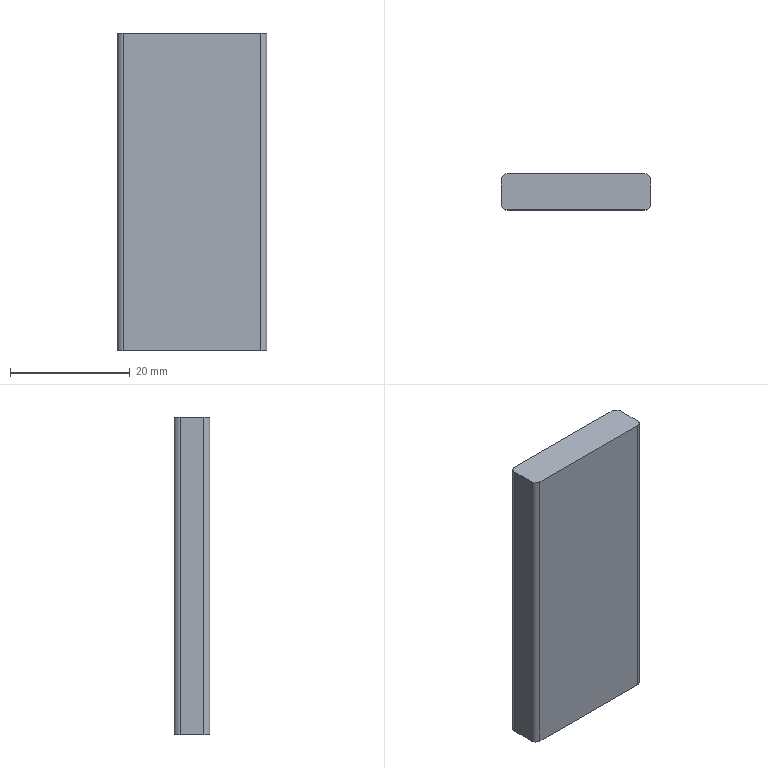Part | STEP file | 200 mesh_id34_xmt | 1 solid | 10 faces | box 24.97 x 5.97 x 53 mm | volume 7855 mm3 | plane 6 | cylinder 4 | commonest cylinder face diameters 2 x4
STEP:
#1=CARTESIAN_POINT('',(-16661.899,-4074.154,0.2));
#2=VERTEX_POINT('',#1);
#3=CARTESIAN_POINT('',(-16684.869,-4074.154,0.2));
#4=VERTEX_POINT('',#3);
#5=CARTESIAN_POINT('',(-16660.884,-4074.154,0.2));
#6=DIRECTION('',(-1.,0.,0.));
#7=VECTOR('',#6,1.);
#8=LINE('',#5,#7);
#9=EDGE_CURVE('',#2,#4,#8,.T.);
#10=ORIENTED_EDGE('',*,*,#9,.T.);
#11=CARTESIAN_POINT('',(-16685.869,-4073.154,0.2));
#12=VERTEX_POINT('',#11);
#13=CARTESIAN_POINT('',(-16684.869,-4073.154,0.2));
#14=DIRECTION('',(0.,0.,-1.));
#15=DIRECTION('',(-1.,0.,0.));
#16=AXIS2_PLACEMENT_3D('',#13,#14,#15);
#17=CIRCLE('',#16,1.);
#18=EDGE_CURVE('',#4,#12,#17,.T.);
#19=ORIENTED_EDGE('',*,*,#18,.T.);
#20=CARTESIAN_POINT('',(-16685.869,-4069.184,0.2));
#21=VERTEX_POINT('',#20);
#22=CARTESIAN_POINT('',(-16685.869,-4074.169,0.2));
#23=DIRECTION('',(0.,1.,0.));
#24=VECTOR('',#23,1.);
#25=LINE('',#22,#24);
#26=EDGE_CURVE('',#12,#21,#25,.T.);
#27=ORIENTED_EDGE('',*,*,#26,.T.);
#28=CARTESIAN_POINT('',(-16684.869,-4068.184,0.2));
#29=VERTEX_POINT('',#28);
#30=CARTESIAN_POINT('',(-16684.869,-4069.184,0.2));
#31=DIRECTION('',(0.,0.,-1.));
#32=DIRECTION('',(-1.,0.,0.));
#33=AXIS2_PLACEMENT_3D('',#30,#31,#32);
#34=CIRCLE('',#33,1.);
#35=EDGE_CURVE('',#21,#29,#34,.T.);
#36=ORIENTED_EDGE('',*,*,#35,.T.);
#37=CARTESIAN_POINT('',(-16661.899,-4068.184,0.2));
#38=VERTEX_POINT('',#37);
#39=CARTESIAN_POINT('',(-16690.884,-4068.184,0.2));
#40=DIRECTION('',(1.,0.,0.));
#41=VECTOR('',#40,1.);
#42=LINE('',#39,#41);
#43=EDGE_CURVE('',#29,#38,#42,.T.);
#44=ORIENTED_EDGE('',*,*,#43,.T.);
#45=CARTESIAN_POINT('',(-16660.899,-4069.184,0.2));
#46=VERTEX_POINT('',#45);
#47=CARTESIAN_POINT('',(-16661.899,-4069.184,0.2));
#48=DIRECTION('',(0.,0.,-1.));
#49=DIRECTION('',(-1.,0.,0.));
#50=AXIS2_PLACEMENT_3D('',#47,#48,#49);
#51=CIRCLE('',#50,1.);
#52=EDGE_CURVE('',#38,#46,#51,.T.);
#53=ORIENTED_EDGE('',*,*,#52,.T.);
#54=CARTESIAN_POINT('',(-16660.899,-4073.154,0.2));
#55=VERTEX_POINT('',#54);
#56=CARTESIAN_POINT('',(-16660.899,-4068.169,0.2));
#57=DIRECTION('',(0.,-1.,0.));
#58=VECTOR('',#57,1.);
#59=LINE('',#56,#58);
#60=EDGE_CURVE('',#46,#55,#59,.T.);
#61=ORIENTED_EDGE('',*,*,#60,.T.);
#62=CARTESIAN_POINT('',(-16661.899,-4073.154,0.2));
#63=DIRECTION('',(0.,0.,-1.));
#64=DIRECTION('',(-1.,0.,0.));
#65=AXIS2_PLACEMENT_3D('',#62,#63,#64);
#66=CIRCLE('',#65,1.);
#67=EDGE_CURVE('',#55,#2,#66,.T.);
#68=ORIENTED_EDGE('',*,*,#67,.T.);
#69=EDGE_LOOP('',(#10,#19,#27,#36,#44,#53,#61,#68));
#70=FACE_OUTER_BOUND('',#69,.T.);
#71=CARTESIAN_POINT('',(2741.269,-60.31,0.2));
#72=DIRECTION('',(0.,0.,-1.));
#73=DIRECTION('',(-1.,0.,0.));
#74=AXIS2_PLACEMENT_3D('',#71,#72,#73);
#75=PLANE('',#74);
#76=ADVANCED_FACE('',(#70),#75,.T.);
#77=CARTESIAN_POINT('',(-16661.899,-4074.154,53.2));
#78=VERTEX_POINT('',#77);
#79=CARTESIAN_POINT('',(-16684.869,-4074.154,53.2));
#80=VERTEX_POINT('',#79);
#81=CARTESIAN_POINT('',(-16660.884,-4074.154,53.2));
#82=DIRECTION('',(-1.,0.,0.));
#83=VECTOR('',#82,1.);
#84=LINE('',#81,#83);
#85=EDGE_CURVE('',#78,#80,#84,.T.);
#86=ORIENTED_EDGE('',*,*,#85,.T.);
#87=CARTESIAN_POINT('',(-16684.869,-4074.154,-382.5));
#88=DIRECTION('',(0.,0.,-1.));
#89=VECTOR('',#88,1.);
#90=LINE('',#87,#89);
#91=EDGE_CURVE('',#80,#4,#90,.T.);
#92=ORIENTED_EDGE('',*,*,#91,.T.);
#93=ORIENTED_EDGE('',*,*,#9,.F.);
#94=CARTESIAN_POINT('',(-16661.899,-4074.154,-382.5));
#95=DIRECTION('',(0.,0.,1.));
#96=VECTOR('',#95,1.);
#97=LINE('',#94,#96);
#98=EDGE_CURVE('',#2,#78,#97,.T.);
#99=ORIENTED_EDGE('',*,*,#98,.T.);
#100=EDGE_LOOP('',(#86,#92,#93,#99));
#101=FACE_OUTER_BOUND('',#100,.T.);
#102=CARTESIAN_POINT('',(-16660.884,-4074.154,-382.5));
#103=DIRECTION('',(0.,1.,0.));
#104=DIRECTION('',(0.,0.,1.));
#105=AXIS2_PLACEMENT_3D('',#102,#103,#104);
#106=PLANE('',#105);
#107=ADVANCED_FACE('',(#101),#106,.F.);
#108=ORIENTED_EDGE('',*,*,#26,.F.);
#109=CARTESIAN_POINT('',(-16685.869,-4073.154,53.2));
#110=VERTEX_POINT('',#109);
#111=CARTESIAN_POINT('',(-16685.869,-4073.154,-382.5));
#112=DIRECTION('',(0.,0.,1.));
#113=VECTOR('',#112,1.);
#114=LINE('',#111,#113);
#115=EDGE_CURVE('',#12,#110,#114,.T.);
#116=ORIENTED_EDGE('',*,*,#115,.T.);
#117=CARTESIAN_POINT('',(-16685.869,-4069.184,53.2));
#118=VERTEX_POINT('',#117);
#119=CARTESIAN_POINT('',(-16685.869,-4074.169,53.2));
#120=DIRECTION('',(0.,1.,0.));
#121=VECTOR('',#120,1.);
#122=LINE('',#119,#121);
#123=EDGE_CURVE('',#110,#118,#122,.T.);
#124=ORIENTED_EDGE('',*,*,#123,.T.);
#125=CARTESIAN_POINT('',(-16685.869,-4069.184,-382.5));
#126=DIRECTION('',(0.,0.,-1.));
#127=VECTOR('',#126,1.);
#128=LINE('',#125,#127);
#129=EDGE_CURVE('',#118,#21,#128,.T.);
#130=ORIENTED_EDGE('',*,*,#129,.T.);
#131=EDGE_LOOP('',(#108,#116,#124,#130));
#132=FACE_OUTER_BOUND('',#131,.T.);
#133=CARTESIAN_POINT('',(-16685.869,-4074.169,-382.5));
#134=DIRECTION('',(1.,0.,0.));
#135=DIRECTION('',(0.,0.,-1.));
#136=AXIS2_PLACEMENT_3D('',#133,#134,#135);
#137=PLANE('',#136);
#138=ADVANCED_FACE('',(#132),#137,.F.);
#139=ORIENTED_EDGE('',*,*,#43,.F.);
#140=CARTESIAN_POINT('',(-16684.869,-4068.184,53.2));
#141=VERTEX_POINT('',#140);
#142=CARTESIAN_POINT('',(-16684.869,-4068.184,-382.5));
#143=DIRECTION('',(0.,0.,1.));
#144=VECTOR('',#143,1.);
#145=LINE('',#142,#144);
#146=EDGE_CURVE('',#29,#141,#145,.T.);
#147=ORIENTED_EDGE('',*,*,#146,.T.);
#148=CARTESIAN_POINT('',(-16661.899,-4068.184,53.2));
#149=VERTEX_POINT('',#148);
#150=CARTESIAN_POINT('',(-16690.884,-4068.184,53.2));
#151=DIRECTION('',(1.,0.,0.));
#152=VECTOR('',#151,1.);
#153=LINE('',#150,#152);
#154=EDGE_CURVE('',#141,#149,#153,.T.);
#155=ORIENTED_EDGE('',*,*,#154,.T.);
#156=CARTESIAN_POINT('',(-16661.899,-4068.184,-382.5));
#157=DIRECTION('',(0.,0.,-1.));
#158=VECTOR('',#157,1.);
#159=LINE('',#156,#158);
#160=EDGE_CURVE('',#149,#38,#159,.T.);
#161=ORIENTED_EDGE('',*,*,#160,.T.);
#162=EDGE_LOOP('',(#139,#147,#155,#161));
#163=FACE_OUTER_BOUND('',#162,.T.);
#164=CARTESIAN_POINT('',(-16690.884,-4068.184,-382.5));
#165=DIRECTION('',(0.,-1.,0.));
#166=DIRECTION('',(0.,0.,-1.));
#167=AXIS2_PLACEMENT_3D('',#164,#165,#166);
#168=PLANE('',#167);
#169=ADVANCED_FACE('',(#163),#168,.F.);
#170=CARTESIAN_POINT('',(-16660.899,-4069.184,53.2));
#171=VERTEX_POINT('',#170);
#172=CARTESIAN_POINT('',(-16660.899,-4073.154,53.2));
#173=VERTEX_POINT('',#172);
#174=CARTESIAN_POINT('',(-16660.899,-4068.169,53.2));
#175=DIRECTION('',(0.,-1.,0.));
#176=VECTOR('',#175,1.);
#177=LINE('',#174,#176);
#178=EDGE_CURVE('',#171,#173,#177,.T.);
#179=ORIENTED_EDGE('',*,*,#178,.T.);
#180=CARTESIAN_POINT('',(-16660.899,-4073.154,-382.5));
#181=DIRECTION('',(0.,0.,-1.));
#182=VECTOR('',#181,1.);
#183=LINE('',#180,#182);
#184=EDGE_CURVE('',#173,#55,#183,.T.);
#185=ORIENTED_EDGE('',*,*,#184,.T.);
#186=ORIENTED_EDGE('',*,*,#60,.F.);
#187=CARTESIAN_POINT('',(-16660.899,-4069.184,-382.5));
#188=DIRECTION('',(0.,0.,1.));
#189=VECTOR('',#188,1.);
#190=LINE('',#187,#189);
#191=EDGE_CURVE('',#46,#171,#190,.T.);
#192=ORIENTED_EDGE('',*,*,#191,.T.);
#193=EDGE_LOOP('',(#179,#185,#186,#192));
#194=FACE_OUTER_BOUND('',#193,.T.);
#195=CARTESIAN_POINT('',(-16660.899,-4068.169,-382.5));
#196=DIRECTION('',(-1.,0.,0.));
#197=DIRECTION('',(0.,0.,1.));
#198=AXIS2_PLACEMENT_3D('',#195,#196,#197);
#199=PLANE('',#198);
#200=ADVANCED_FACE('',(#194),#199,.F.);
#201=ORIENTED_EDGE('',*,*,#123,.F.);
#202=CARTESIAN_POINT('',(-16684.869,-4073.154,53.2));
#203=DIRECTION('',(0.,0.,1.));
#204=DIRECTION('',(-1.,0.,0.));
#205=AXIS2_PLACEMENT_3D('',#202,#203,#204);
#206=CIRCLE('',#205,1.);
#207=EDGE_CURVE('',#110,#80,#206,.T.);
#208=ORIENTED_EDGE('',*,*,#207,.T.);
#209=ORIENTED_EDGE('',*,*,#85,.F.);
#210=CARTESIAN_POINT('',(-16661.899,-4073.154,53.2));
#211=DIRECTION('',(0.,0.,1.));
#212=DIRECTION('',(-1.,0.,0.));
#213=AXIS2_PLACEMENT_3D('',#210,#211,#212);
#214=CIRCLE('',#213,1.);
#215=EDGE_CURVE('',#78,#173,#214,.T.);
#216=ORIENTED_EDGE('',*,*,#215,.T.);
#217=ORIENTED_EDGE('',*,*,#178,.F.);
#218=CARTESIAN_POINT('',(-16661.899,-4069.184,53.2));
#219=DIRECTION('',(0.,0.,1.));
#220=DIRECTION('',(-1.,0.,0.));
#221=AXIS2_PLACEMENT_3D('',#218,#219,#220);
#222=CIRCLE('',#221,1.);
#223=EDGE_CURVE('',#171,#149,#222,.T.);
#224=ORIENTED_EDGE('',*,*,#223,.T.);
#225=ORIENTED_EDGE('',*,*,#154,.F.);
#226=CARTESIAN_POINT('',(-16684.869,-4069.184,53.2));
#227=DIRECTION('',(0.,0.,1.));
#228=DIRECTION('',(-1.,0.,0.));
#229=AXIS2_PLACEMENT_3D('',#226,#227,#228);
#230=CIRCLE('',#229,1.);
#231=EDGE_CURVE('',#141,#118,#230,.T.);
#232=ORIENTED_EDGE('',*,*,#231,.T.);
#233=EDGE_LOOP('',(#201,#208,#209,#216,#217,#224,#225,#232));
#234=FACE_OUTER_BOUND('',#233,.T.);
#235=CARTESIAN_POINT('',(504.,-60.31,53.2));
#236=DIRECTION('',(0.,0.,-1.));
#237=DIRECTION('',(-1.,0.,0.));
#238=AXIS2_PLACEMENT_3D('',#235,#236,#237);
#239=PLANE('',#238);
#240=ADVANCED_FACE('',(#234),#239,.F.);
#241=ORIENTED_EDGE('',*,*,#18,.F.);
#242=ORIENTED_EDGE('',*,*,#91,.F.);
#243=ORIENTED_EDGE('',*,*,#207,.F.);
#244=ORIENTED_EDGE('',*,*,#115,.F.);
#245=EDGE_LOOP('',(#241,#242,#243,#244));
#246=FACE_OUTER_BOUND('',#245,.T.);
#247=CARTESIAN_POINT('',(-16684.869,-4073.154,-382.5));
#248=DIRECTION('',(0.,0.,1.));
#249=DIRECTION('',(1.,0.,0.));
#250=AXIS2_PLACEMENT_3D('',#247,#248,#249);
#251=CYLINDRICAL_SURFACE('',#250,1.);
#252=ADVANCED_FACE('',(#246),#251,.T.);
#253=ORIENTED_EDGE('',*,*,#35,.F.);
#254=ORIENTED_EDGE('',*,*,#129,.F.);
#255=ORIENTED_EDGE('',*,*,#231,.F.);
#256=ORIENTED_EDGE('',*,*,#146,.F.);
#257=EDGE_LOOP('',(#253,#254,#255,#256));
#258=FACE_OUTER_BOUND('',#257,.T.);
#259=CARTESIAN_POINT('',(-16684.869,-4069.184,-382.5));
#260=DIRECTION('',(0.,0.,1.));
#261=DIRECTION('',(1.,0.,0.));
#262=AXIS2_PLACEMENT_3D('',#259,#260,#261);
#263=CYLINDRICAL_SURFACE('',#262,1.);
#264=ADVANCED_FACE('',(#258),#263,.T.);
#265=ORIENTED_EDGE('',*,*,#67,.F.);
#266=ORIENTED_EDGE('',*,*,#184,.F.);
#267=ORIENTED_EDGE('',*,*,#215,.F.);
#268=ORIENTED_EDGE('',*,*,#98,.F.);
#269=EDGE_LOOP('',(#265,#266,#267,#268));
#270=FACE_OUTER_BOUND('',#269,.T.);
#271=CARTESIAN_POINT('',(-16661.899,-4073.154,-382.5));
#272=DIRECTION('',(0.,0.,1.));
#273=DIRECTION('',(1.,0.,0.));
#274=AXIS2_PLACEMENT_3D('',#271,#272,#273);
#275=CYLINDRICAL_SURFACE('',#274,1.);
#276=ADVANCED_FACE('',(#270),#275,.T.);
#277=ORIENTED_EDGE('',*,*,#52,.F.);
#278=ORIENTED_EDGE('',*,*,#160,.F.);
#279=ORIENTED_EDGE('',*,*,#223,.F.);
#280=ORIENTED_EDGE('',*,*,#191,.F.);
#281=EDGE_LOOP('',(#277,#278,#279,#280));
#282=FACE_OUTER_BOUND('',#281,.T.);
#283=CARTESIAN_POINT('',(-16661.899,-4069.184,-382.5));
#284=DIRECTION('',(0.,0.,1.));
#285=DIRECTION('',(1.,0.,0.));
#286=AXIS2_PLACEMENT_3D('',#283,#284,#285);
#287=CYLINDRICAL_SURFACE('',#286,1.);
#288=ADVANCED_FACE('',(#282),#287,.T.);
#289=CLOSED_SHELL('',(#76,#107,#138,#169,#200,#240,#252,#264,#276,#288));
#290=MANIFOLD_SOLID_BREP('',#289);
#291=(LENGTH_UNIT()NAMED_UNIT(*)SI_UNIT(.MILLI.,.METRE.));
#292=UNCERTAINTY_MEASURE_WITH_UNIT(LENGTH_MEASURE(0.00002),#291,'','');
#293=(NAMED_UNIT(*)PLANE_ANGLE_UNIT()SI_UNIT($,.RADIAN.));
#294=PLANE_ANGLE_MEASURE_WITH_UNIT(PLANE_ANGLE_MEASURE(0.01745),#293);
#295=DIMENSIONAL_EXPONENTS(0.,0.,0.,0.,0.,0.,0.);
#296=(CONVERSION_BASED_UNIT('DEGREE',#294)NAMED_UNIT(#295)PLANE_ANGLE_UNIT());
#297=(NAMED_UNIT(*)SI_UNIT($,.STERADIAN.)SOLID_ANGLE_UNIT());
#298=(GEOMETRIC_REPRESENTATION_CONTEXT(3)GLOBAL_UNCERTAINTY_ASSIGNED_CONTEXT((#292))GLOBAL_UNIT_ASSIGNED_CONTEXT((#291,#296,#297))REPRESENTATION_CONTEXT('',''));
#299=ADVANCED_BREP_SHAPE_REPRESENTATION('',(#290),#298);